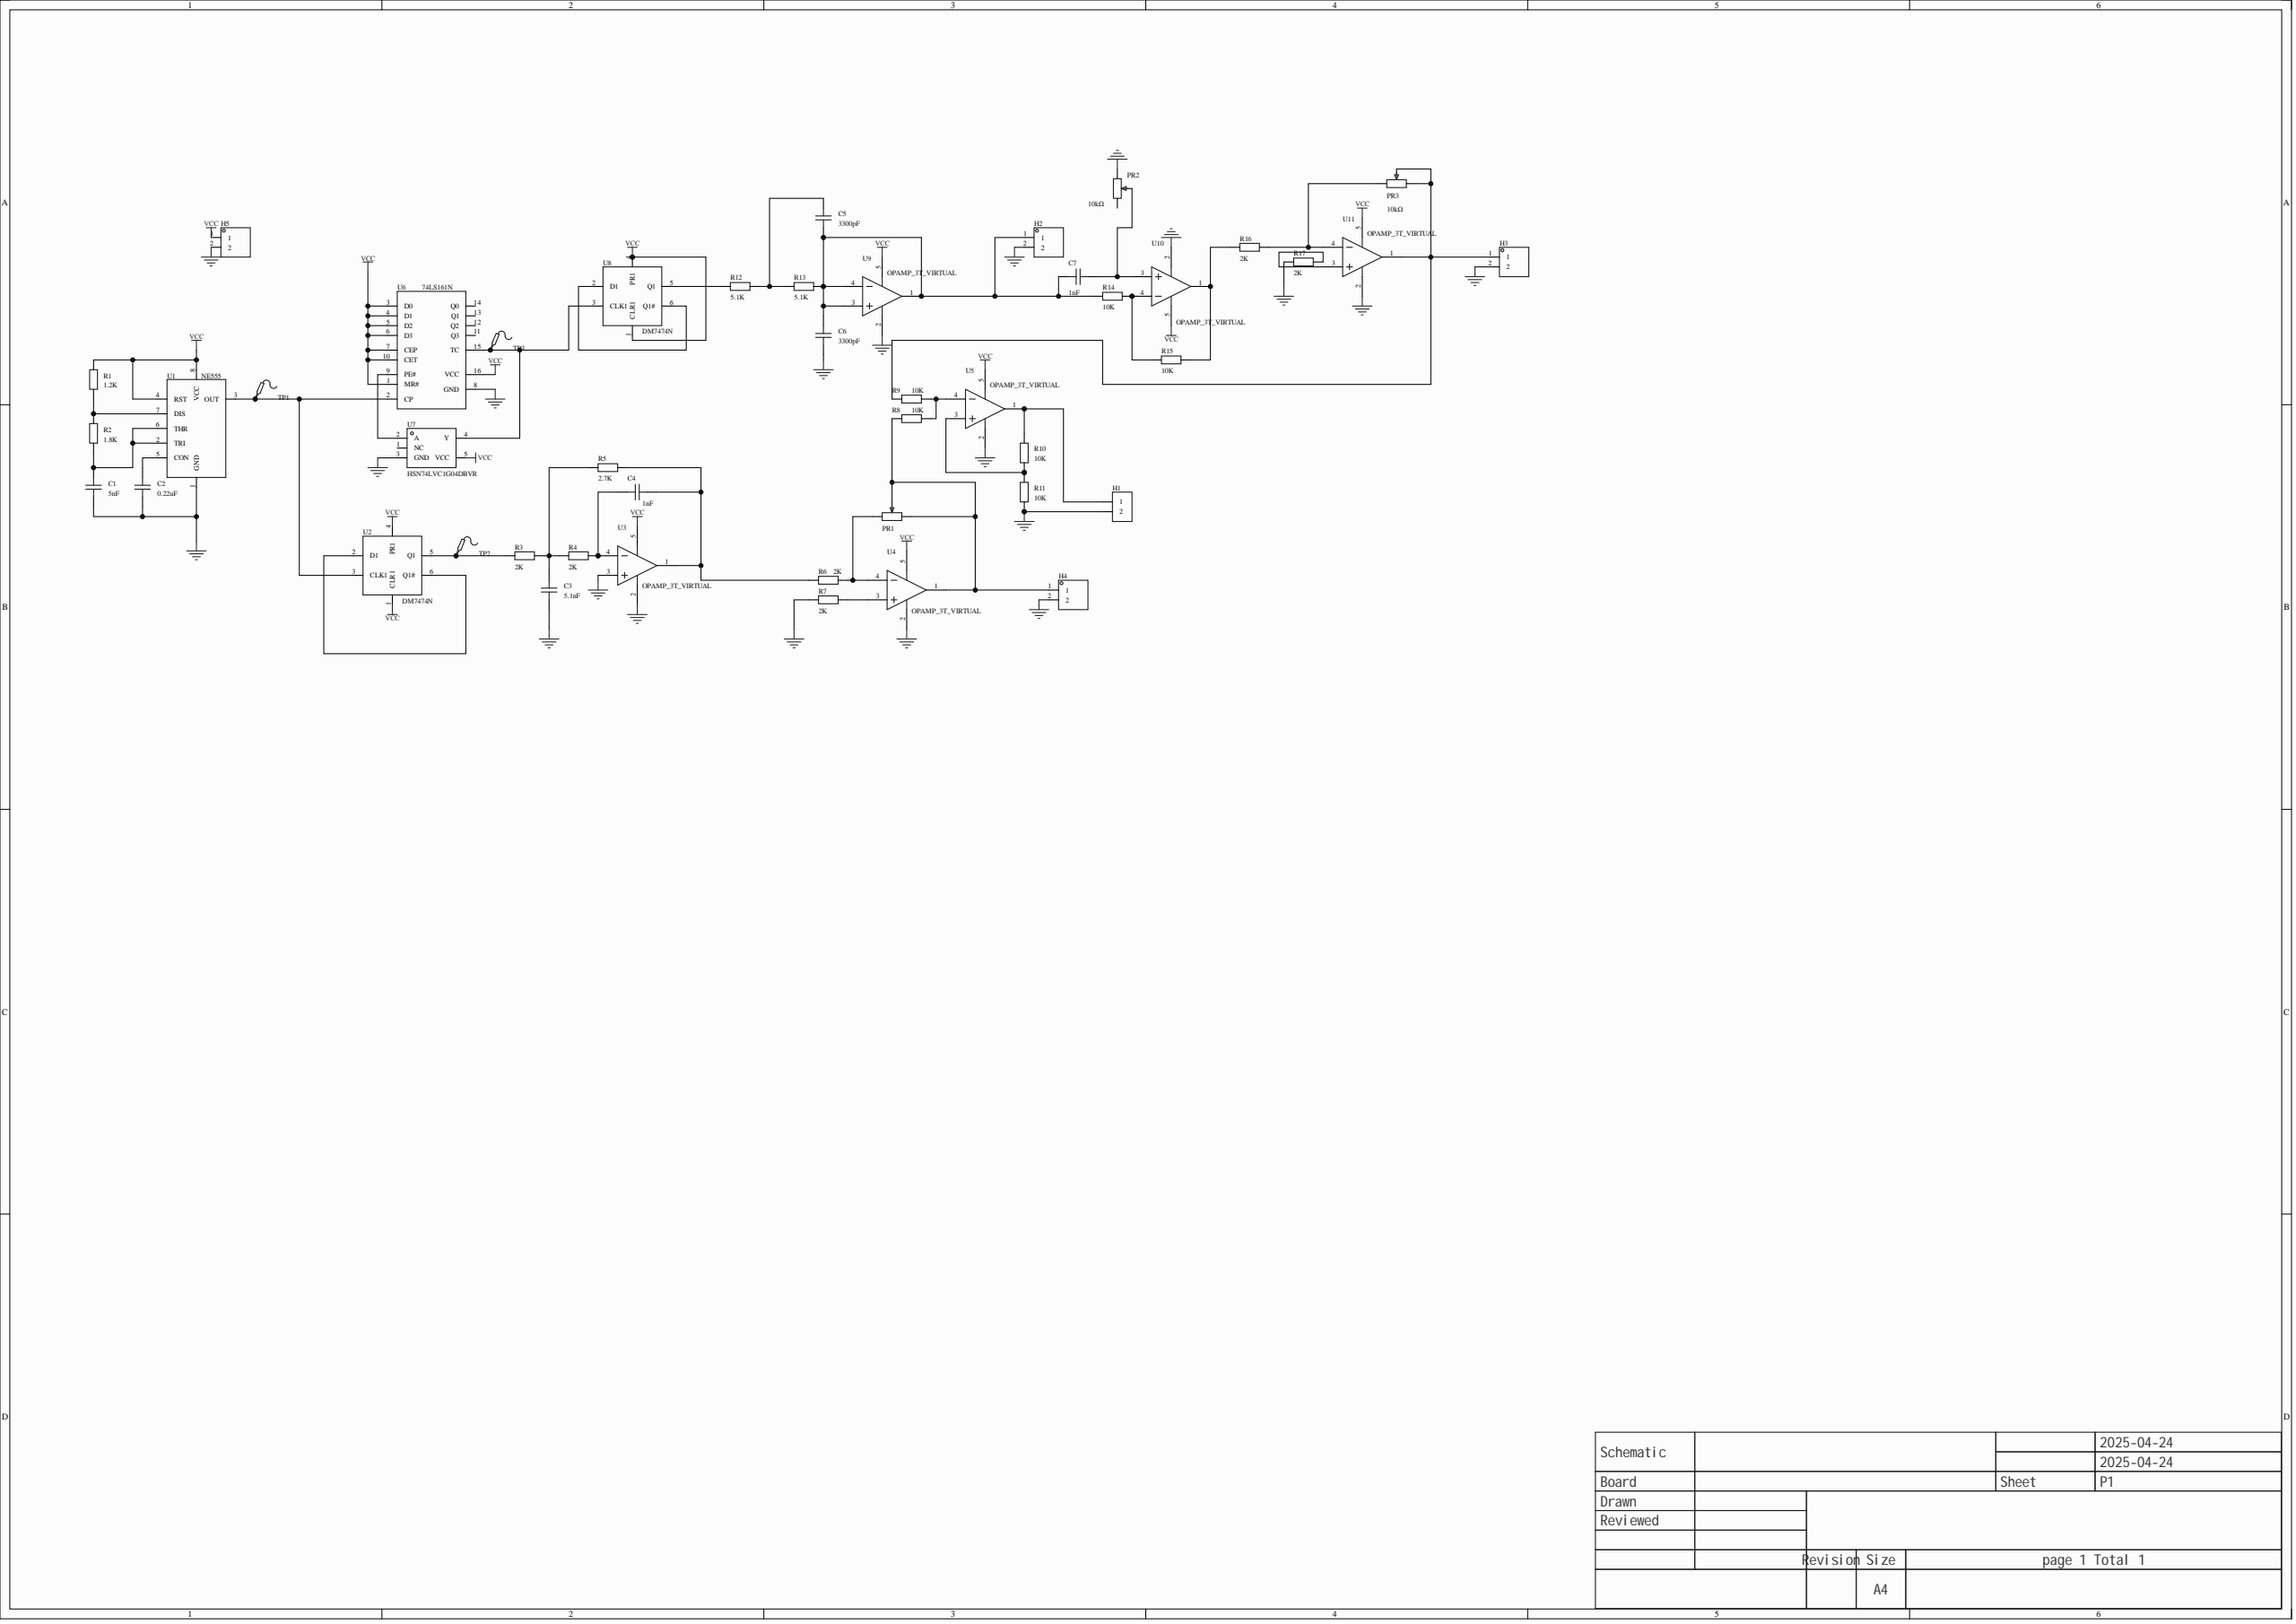Circuit board | Altium Designer | 46 parts | 29 nets
Bill of materials:
Comment,Description,Designator,Footprint,LibRef,Quantity
"5nF","","C1","C0603","CAP_0603","1"
"0.22uF","","C2","C0603","CAP_0603","1"
"5.1nF","","C3","C0603","CAP_0603","1"
"1nF","","C4, C7","C0603","CAP_0603","2"
"3300pF","","C5, C6","C0603","CAP_0603","2"
"","","H1","HDR-TH_2P-P2.54-V-F","HDR-F_2.54_1x2P","1"
"","","H2, H3, H4, H5","HDR-TH_2P-P2.54-V-M-1","HDR-M_2.54_1x2P","4"
"10kΩ","","PR1, PR2, PR3","R_3296","R_3296","3"
"1.2K","","R1","R0603","Res_0603","1"
"1.8K","","R2","R0603","Res_0603","1"
"2K","","R3, R4, R6, R7, R16, R17","R0603","Res_0603","6"
"2.7K","","R5","R0603","Res_0603","1"
"10K","","R8, R9, R10, R11, R14, R15","R0603","Res_0603","6"
"5.1K","","R12, R13","R0603","Res_0603","2"
"","Test Point","TP1, TP2, TP3","Test-Point-0.5mm","Test-Point","3"
"NE555","NE555 single-precision timer","U1","PDIP-8_L9.6-W6.4-P2.54-LS7.9-BL-1","NE555PE4","1"
"DM7474N","Type: D-type; supply voltage: 4.75V~5.25V; clock frequency: 15MHz; elements: 2; bits per element: 1; max propagation delay: 40ns@5V,15pF; quiescent current (Iq): 30mA;","U2, U8","PDIP-14_L19.5-W6.7-P2.54-LS7.9-BL","DM7474N","2"
"OPAMP_3T_VIRTUAL","","U3, U4, U5, U9, U10, U11","SOT-23-5_L3.0-W1.7-P0.95-LS2.8-BR","OPA376AIDBVOPAMPSOT23-5","6"
"74LS161N","Operating voltage: 2V~6V; elements: 1; trigger edge: rising edge; count rate: 27MHz;","U6","PDIP-16_L19.3-W6.4-P2.54-LS7.94-BL","SN74LS161N(LX)","1"
"HSN74LVC1G04DBVR","Logic type: inverter; channels: 1; operating voltage: 1.65V~5.5V; quiescent current (Iq): 10uA;","U7","SOT-23-5_L2.9-W1.6-P0.95-LS2.9-BL","HSN74LVC1G04DBVR","1"
Netlist (Protel format):
[
C1
C0603
5nF



]
[
C2
C0603
0.22uF



]
[
C3
C0603
5.1nF



]
[
C4
C0603
1nF



]
[
C5
C0603
3300pF



]
[
C6
C0603
3300pF



]
[
C7
C0603
1nF



]
[
H1
HDR-TH_2P-P2.54-V-F




]
[
H2
HDR-TH_2P-P2.54-V-M-1




]
[
H3
HDR-TH_2P-P2.54-V-M-1




]
[
H4
HDR-TH_2P-P2.54-V-M-1




]
[
H5
HDR-TH_2P-P2.54-V-M-1




]
[
PR1
R_3296
10kΩ



]
[
PR2
R_3296
10kΩ



]
[
PR3
R_3296
10kΩ



]
[
R1
R0603
1.2K



]
[
R2
R0603
1.8K



]
[
R3
R0603
2K



]
[
R4
R0603
2K



]
[
R5
R0603
2.7K



]
[
R6
R0603
2K



]
[
R7
R0603
2K



]
[
R8
R0603
10K



]
[
R9
R0603
10K



]
[
R10
R0603
10K



]
[
R11
R0603
10K



]
[
R12
R0603
5.1K



]
[
R13
R0603
5.1K



]
[
R14
R0603
10K



]
[
R15
R0603
10K



]
[
R16
R0603
2K



]
[
R17
R0603
2K



]
[
TP1
Test-Point-0.5mm




]
[
TP2
Test-Point-0.5mm




]
[
TP3
Test-Point-0.5mm




]
[
U1
PDIP-8_L9.6-W6.4-P2.54-LS7.9-BL-1
NE555



]
[
U2
PDIP-14_L19.5-W6.7-P2.54-LS7.9-BL
DM7474N



]
[
U3
SOT-23-5_L3.0-W1.7-P0.95-LS2.8-BR
OPAMP_3T_VIRTUAL



]
[
U4
SOT-23-5_L3.0-W1.7-P0.95-LS2.8-BR
OPAMP_3T_VIRTUAL



]
[
U5
SOT-23-5_L3.0-W1.7-P0.95-LS2.8-BR
OPAMP_3T_VIRTUAL



]
[
U6
PDIP-16_L19.3-W6.4-P2.54-LS7.94-BL
74LS161N



]
[
U7
SOT-23-5_L2.9-W1.6-P0.95-LS2.9-BL
HSN74LVC1G04DBVR



]
[
U8
PDIP-14_L19.5-W6.7-P2.54-LS7.9-BL
DM7474N



]
[
U9
SOT-23-5_L3.0-W1.7-P0.95-LS2.8-BR
OPAMP_3T_VIRTUAL



]
[
U10
SOT-23-5_L3.0-W1.7-P0.95-LS2.8-BR
OPAMP_3T_VIRTUAL



]
[
U11
SOT-23-5_L3.0-W1.7-P0.95-LS2.8-BR
OPAMP_3T_VIRTUAL



]
(
VCC
H5-1
R1-2
U1-4
U1-8
U2-1
U2-4
U3-5
U4-5
U5-5
U6-1
U6-3
U6-4
U6-5
U6-6
U6-7
U6-10
U6-16
U7-5
U8-1
U8-4
U9-5
U10-5
U11-5
)
(
NetU8_2
U8-2
U8-6
)
(
NetU6_9
U6-9
U7-2
)
(
NetU2_2
U2-2
U2-6
)
(
NetTP3_1
TP3-1
U6-15
U7-4
U8-3
)
(
NetTP1_1
TP1-1
U1-3
U2-3
U6-2
)
(
NetR17_2
R17-2
U11-3
)
(
NetR15_2
R15-2
R16-1
U10-1
)
(
NetR14_2
R14-2
R15-1
U10-4
)
(
NetR12_1
R12-1
U8-5
)
(
NetR10_1
R10-1
R11-2
U5-3
)
(
NetR8_2
R8-2
R9-2
U5-4
)
(
NetR7_2
R7-2
U4-3
)
(
NetR3_1
R3-1
TP2-1
U2-5
)
(
NetR1_1
R1-1
R2-2
U1-7
)
(
NetPR3_3
PR3-3
R16-2
U11-4
)
(
NetPR1_3
PR1-3
R6-2
U4-4
)
(
NetH4_1
H4-1
PR1-1
PR1-2
R8-1
U4-1
)
(
NetH3_1
H3-1
PR3-1
PR3-2
R9-1
U11-1
)
(
NetH1_1
H1-1
R10-2
U5-1
)
(
NetC7_1
C7-1
PR2-2
U10-3
)
(
NetC5_2
C5-2
R12-2
R13-1
)
(
NetC5_1
C5-1
C6-2
C7-2
H2-1
R13-2
R14-1
U9-1
U9-3
U9-4
)
(
NetC4_2
C4-2
R5-2
R6-1
U3-1
)
(
NetC4_1
C4-1
R4-2
U3-4
)
(
NetC3_2
C3-2
R3-2
R4-1
R5-1
)
(
NetC2_2
C2-2
U1-5
)
(
NetC1_2
C1-2
R2-1
U1-2
U1-6
)
(
GND
C1-1
C2-1
C3-1
C6-1
H1-2
H2-2
H3-2
H4-2
H5-2
PR2-3
R7-1
R11-1
R17-1
U1-1
U3-2
U3-3
U4-2
U5-2
U6-8
U7-3
U9-2
U10-2
U11-2
)